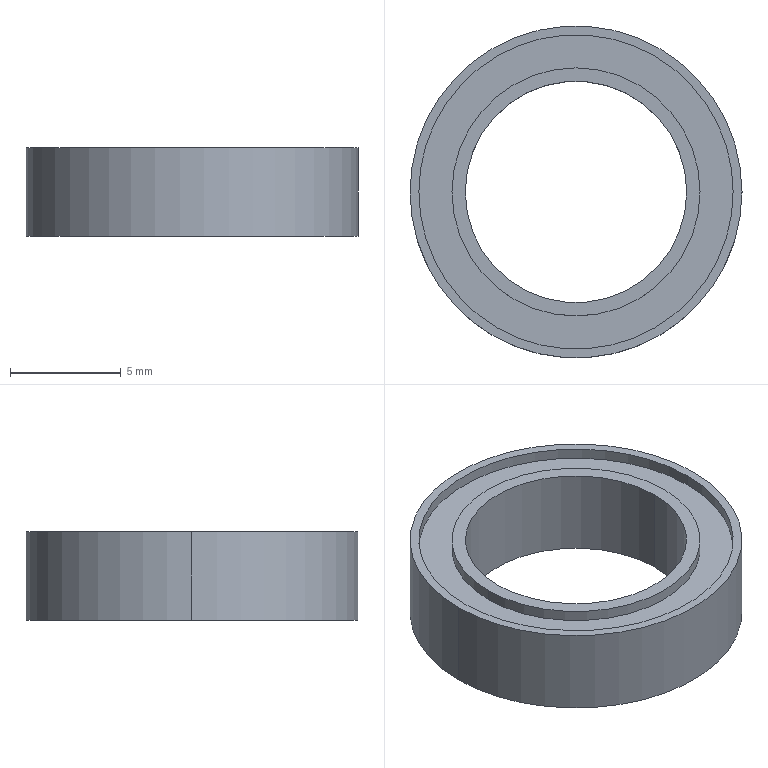Part | SolidWorks | features Extrusion 1, ICE 1, MirrorPattern 1 | 1 solid | 18 faces | box 15 x 15 x 4 mm | volume 333.028 mm3 | cylinder 12 | plane 6 | commonest cylinder face diameters 11.21 x4 14.2 x4 10 x2 15 x2
STEP:
#1=CARTESIAN_POINT('',(5.605,0.,-1.5));
#2=VERTEX_POINT('',#1);
#3=CARTESIAN_POINT('',(-5.605,0.,-1.5));
#4=VERTEX_POINT('',#3);
#5=CARTESIAN_POINT('',(0.,0.,-1.5));
#6=DIRECTION('',(0.,0.,1.));
#7=DIRECTION('',(1.,0.,0.));
#8=AXIS2_PLACEMENT_3D('',#5,#6,#7);
#9=CIRCLE('',#8,5.605);
#10=EDGE_CURVE('',#2,#4,#9,.T.);
#11=ORIENTED_EDGE('',*,*,#10,.F.);
#12=CARTESIAN_POINT('',(5.605,0.,-2.));
#13=VERTEX_POINT('',#12);
#14=CARTESIAN_POINT('',(5.605,0.,-1.5));
#15=DIRECTION('',(0.,0.,-1.));
#16=VECTOR('',#15,1000.);
#17=LINE('',#14,#16);
#18=EDGE_CURVE('',#2,#13,#17,.T.);
#19=ORIENTED_EDGE('',*,*,#18,.T.);
#20=CARTESIAN_POINT('',(-5.605,0.,-2.));
#21=VERTEX_POINT('',#20);
#22=CARTESIAN_POINT('',(0.,0.,-2.));
#23=DIRECTION('',(0.,0.,1.));
#24=DIRECTION('',(1.,0.,0.));
#25=AXIS2_PLACEMENT_3D('',#22,#23,#24);
#26=CIRCLE('',#25,5.605);
#27=EDGE_CURVE('',#13,#21,#26,.T.);
#28=ORIENTED_EDGE('',*,*,#27,.T.);
#29=CARTESIAN_POINT('',(-5.605,0.,-1.5));
#30=DIRECTION('',(0.,0.,-1.));
#31=VECTOR('',#30,1000.);
#32=LINE('',#29,#31);
#33=EDGE_CURVE('',#4,#21,#32,.T.);
#34=ORIENTED_EDGE('',*,*,#33,.F.);
#35=EDGE_LOOP('',(#11,#19,#28,#34));
#36=FACE_OUTER_BOUND('',#35,.T.);
#37=CARTESIAN_POINT('',(0.,0.,-1.5));
#38=DIRECTION('',(0.,0.,-1.));
#39=DIRECTION('',(-1.,0.,0.));
#40=AXIS2_PLACEMENT_3D('',#37,#38,#39);
#41=CYLINDRICAL_SURFACE('',#40,5.605);
#42=ADVANCED_FACE('',(#36),#41,.T.);
#43=CARTESIAN_POINT('',(-7.1,0.,-1.5));
#44=VERTEX_POINT('',#43);
#45=CARTESIAN_POINT('',(7.1,0.,-1.5));
#46=VERTEX_POINT('',#45);
#47=CARTESIAN_POINT('',(0.,0.,-1.5));
#48=DIRECTION('',(0.,0.,1.));
#49=DIRECTION('',(1.,0.,0.));
#50=AXIS2_PLACEMENT_3D('',#47,#48,#49);
#51=CIRCLE('',#50,7.1);
#52=EDGE_CURVE('',#44,#46,#51,.T.);
#53=ORIENTED_EDGE('',*,*,#52,.T.);
#54=CARTESIAN_POINT('',(7.1,0.,-2.));
#55=VERTEX_POINT('',#54);
#56=CARTESIAN_POINT('',(7.1,0.,-1.5));
#57=DIRECTION('',(0.,0.,-1.));
#58=VECTOR('',#57,1000.);
#59=LINE('',#56,#58);
#60=EDGE_CURVE('',#46,#55,#59,.T.);
#61=ORIENTED_EDGE('',*,*,#60,.T.);
#62=CARTESIAN_POINT('',(-7.1,0.,-2.));
#63=VERTEX_POINT('',#62);
#64=CARTESIAN_POINT('',(0.,0.,-2.));
#65=DIRECTION('',(0.,0.,1.));
#66=DIRECTION('',(1.,0.,0.));
#67=AXIS2_PLACEMENT_3D('',#64,#65,#66);
#68=CIRCLE('',#67,7.1);
#69=EDGE_CURVE('',#63,#55,#68,.T.);
#70=ORIENTED_EDGE('',*,*,#69,.F.);
#71=CARTESIAN_POINT('',(-7.1,0.,-1.5));
#72=DIRECTION('',(0.,0.,-1.));
#73=VECTOR('',#72,1000.);
#74=LINE('',#71,#73);
#75=EDGE_CURVE('',#44,#63,#74,.T.);
#76=ORIENTED_EDGE('',*,*,#75,.F.);
#77=EDGE_LOOP('',(#53,#61,#70,#76));
#78=FACE_OUTER_BOUND('',#77,.T.);
#79=CARTESIAN_POINT('',(0.,0.,-1.5));
#80=DIRECTION('',(0.,0.,-1.));
#81=DIRECTION('',(-1.,0.,0.));
#82=AXIS2_PLACEMENT_3D('',#79,#80,#81);
#83=CYLINDRICAL_SURFACE('',#82,7.1);
#84=ADVANCED_FACE('',(#78),#83,.F.);
#85=CARTESIAN_POINT('',(5.605,0.,1.5));
#86=VERTEX_POINT('',#85);
#87=CARTESIAN_POINT('',(-5.605,0.,1.5));
#88=VERTEX_POINT('',#87);
#89=CARTESIAN_POINT('',(0.,0.,1.5));
#90=DIRECTION('',(0.,0.,1.));
#91=DIRECTION('',(1.,0.,0.));
#92=AXIS2_PLACEMENT_3D('',#89,#90,#91);
#93=CIRCLE('',#92,5.605);
#94=EDGE_CURVE('',#86,#88,#93,.T.);
#95=ORIENTED_EDGE('',*,*,#94,.T.);
#96=CARTESIAN_POINT('',(-5.605,0.,2.));
#97=VERTEX_POINT('',#96);
#98=CARTESIAN_POINT('',(-5.605,0.,1.5));
#99=DIRECTION('',(0.,0.,1.));
#100=VECTOR('',#99,1000.);
#101=LINE('',#98,#100);
#102=EDGE_CURVE('',#88,#97,#101,.T.);
#103=ORIENTED_EDGE('',*,*,#102,.T.);
#104=CARTESIAN_POINT('',(5.605,0.,2.));
#105=VERTEX_POINT('',#104);
#106=CARTESIAN_POINT('',(0.,0.,2.));
#107=DIRECTION('',(0.,0.,1.));
#108=DIRECTION('',(1.,0.,0.));
#109=AXIS2_PLACEMENT_3D('',#106,#107,#108);
#110=CIRCLE('',#109,5.605);
#111=EDGE_CURVE('',#105,#97,#110,.T.);
#112=ORIENTED_EDGE('',*,*,#111,.F.);
#113=CARTESIAN_POINT('',(5.605,0.,1.5));
#114=DIRECTION('',(0.,0.,1.));
#115=VECTOR('',#114,1000.);
#116=LINE('',#113,#115);
#117=EDGE_CURVE('',#86,#105,#116,.T.);
#118=ORIENTED_EDGE('',*,*,#117,.F.);
#119=EDGE_LOOP('',(#95,#103,#112,#118));
#120=FACE_OUTER_BOUND('',#119,.T.);
#121=CARTESIAN_POINT('',(0.,0.,1.5));
#122=DIRECTION('',(0.,0.,1.));
#123=DIRECTION('',(1.,0.,0.));
#124=AXIS2_PLACEMENT_3D('',#121,#122,#123);
#125=CYLINDRICAL_SURFACE('',#124,5.605);
#126=ADVANCED_FACE('',(#120),#125,.T.);
#127=CARTESIAN_POINT('',(-7.1,0.,1.5));
#128=VERTEX_POINT('',#127);
#129=CARTESIAN_POINT('',(7.1,0.,1.5));
#130=VERTEX_POINT('',#129);
#131=CARTESIAN_POINT('',(0.,0.,1.5));
#132=DIRECTION('',(0.,0.,1.));
#133=DIRECTION('',(1.,0.,0.));
#134=AXIS2_PLACEMENT_3D('',#131,#132,#133);
#135=CIRCLE('',#134,7.1);
#136=EDGE_CURVE('',#128,#130,#135,.T.);
#137=ORIENTED_EDGE('',*,*,#136,.F.);
#138=CARTESIAN_POINT('',(-7.1,0.,2.));
#139=VERTEX_POINT('',#138);
#140=CARTESIAN_POINT('',(-7.1,0.,1.5));
#141=DIRECTION('',(0.,0.,1.));
#142=VECTOR('',#141,1000.);
#143=LINE('',#140,#142);
#144=EDGE_CURVE('',#128,#139,#143,.T.);
#145=ORIENTED_EDGE('',*,*,#144,.T.);
#146=CARTESIAN_POINT('',(7.1,0.,2.));
#147=VERTEX_POINT('',#146);
#148=CARTESIAN_POINT('',(0.,0.,2.));
#149=DIRECTION('',(0.,0.,1.));
#150=DIRECTION('',(1.,0.,0.));
#151=AXIS2_PLACEMENT_3D('',#148,#149,#150);
#152=CIRCLE('',#151,7.1);
#153=EDGE_CURVE('',#139,#147,#152,.T.);
#154=ORIENTED_EDGE('',*,*,#153,.T.);
#155=CARTESIAN_POINT('',(7.1,0.,1.5));
#156=DIRECTION('',(0.,0.,1.));
#157=VECTOR('',#156,1000.);
#158=LINE('',#155,#157);
#159=EDGE_CURVE('',#130,#147,#158,.T.);
#160=ORIENTED_EDGE('',*,*,#159,.F.);
#161=EDGE_LOOP('',(#137,#145,#154,#160));
#162=FACE_OUTER_BOUND('',#161,.T.);
#163=CARTESIAN_POINT('',(0.,0.,1.5));
#164=DIRECTION('',(0.,0.,1.));
#165=DIRECTION('',(1.,0.,0.));
#166=AXIS2_PLACEMENT_3D('',#163,#164,#165);
#167=CYLINDRICAL_SURFACE('',#166,7.1);
#168=ADVANCED_FACE('',(#162),#167,.F.);
#169=CARTESIAN_POINT('',(-5.,0.,-2.));
#170=VERTEX_POINT('',#169);
#171=CARTESIAN_POINT('',(5.,0.,-2.));
#172=VERTEX_POINT('',#171);
#173=CARTESIAN_POINT('',(0.,0.,-2.));
#174=DIRECTION('',(0.,0.,1.));
#175=DIRECTION('',(1.,0.,0.));
#176=AXIS2_PLACEMENT_3D('',#173,#174,#175);
#177=CIRCLE('',#176,5.);
#178=EDGE_CURVE('',#170,#172,#177,.T.);
#179=ORIENTED_EDGE('',*,*,#178,.F.);
#180=CARTESIAN_POINT('',(-5.,0.,2.));
#181=VERTEX_POINT('',#180);
#182=CARTESIAN_POINT('',(-5.,0.,-2.));
#183=DIRECTION('',(0.,0.,1.));
#184=VECTOR('',#183,1000.);
#185=LINE('',#182,#184);
#186=EDGE_CURVE('',#170,#181,#185,.T.);
#187=ORIENTED_EDGE('',*,*,#186,.T.);
#188=CARTESIAN_POINT('',(5.,0.,2.));
#189=VERTEX_POINT('',#188);
#190=CARTESIAN_POINT('',(0.,0.,2.));
#191=DIRECTION('',(0.,0.,1.));
#192=DIRECTION('',(1.,0.,0.));
#193=AXIS2_PLACEMENT_3D('',#190,#191,#192);
#194=CIRCLE('',#193,5.);
#195=EDGE_CURVE('',#181,#189,#194,.T.);
#196=ORIENTED_EDGE('',*,*,#195,.T.);
#197=CARTESIAN_POINT('',(5.,0.,-2.));
#198=DIRECTION('',(0.,0.,1.));
#199=VECTOR('',#198,1000.);
#200=LINE('',#197,#199);
#201=EDGE_CURVE('',#172,#189,#200,.T.);
#202=ORIENTED_EDGE('',*,*,#201,.F.);
#203=EDGE_LOOP('',(#179,#187,#196,#202));
#204=FACE_OUTER_BOUND('',#203,.T.);
#205=CARTESIAN_POINT('',(0.,0.,-2.));
#206=DIRECTION('',(0.,0.,1.));
#207=DIRECTION('',(1.,0.,0.));
#208=AXIS2_PLACEMENT_3D('',#205,#206,#207);
#209=CYLINDRICAL_SURFACE('',#208,5.);
#210=ADVANCED_FACE('',(#204),#209,.F.);
#211=CARTESIAN_POINT('',(7.5,0.,-2.));
#212=VERTEX_POINT('',#211);
#213=CARTESIAN_POINT('',(-7.5,0.,-2.));
#214=VERTEX_POINT('',#213);
#215=CARTESIAN_POINT('',(0.,0.,-2.));
#216=DIRECTION('',(0.,0.,1.));
#217=DIRECTION('',(1.,0.,0.));
#218=AXIS2_PLACEMENT_3D('',#215,#216,#217);
#219=CIRCLE('',#218,7.5);
#220=EDGE_CURVE('',#212,#214,#219,.T.);
#221=ORIENTED_EDGE('',*,*,#220,.T.);
#222=CARTESIAN_POINT('',(-7.5,0.,2.));
#223=VERTEX_POINT('',#222);
#224=CARTESIAN_POINT('',(-7.5,0.,-2.));
#225=DIRECTION('',(0.,0.,1.));
#226=VECTOR('',#225,1000.);
#227=LINE('',#224,#226);
#228=EDGE_CURVE('',#214,#223,#227,.T.);
#229=ORIENTED_EDGE('',*,*,#228,.T.);
#230=CARTESIAN_POINT('',(7.5,0.,2.));
#231=VERTEX_POINT('',#230);
#232=CARTESIAN_POINT('',(0.,0.,2.));
#233=DIRECTION('',(0.,0.,1.));
#234=DIRECTION('',(1.,0.,0.));
#235=AXIS2_PLACEMENT_3D('',#232,#233,#234);
#236=CIRCLE('',#235,7.5);
#237=EDGE_CURVE('',#231,#223,#236,.T.);
#238=ORIENTED_EDGE('',*,*,#237,.F.);
#239=CARTESIAN_POINT('',(7.5,0.,-2.));
#240=DIRECTION('',(0.,0.,1.));
#241=VECTOR('',#240,1000.);
#242=LINE('',#239,#241);
#243=EDGE_CURVE('',#212,#231,#242,.T.);
#244=ORIENTED_EDGE('',*,*,#243,.F.);
#245=EDGE_LOOP('',(#221,#229,#238,#244));
#246=FACE_OUTER_BOUND('',#245,.T.);
#247=CARTESIAN_POINT('',(0.,0.,-2.));
#248=DIRECTION('',(0.,0.,1.));
#249=DIRECTION('',(1.,0.,0.));
#250=AXIS2_PLACEMENT_3D('',#247,#248,#249);
#251=CYLINDRICAL_SURFACE('',#250,7.5);
#252=ADVANCED_FACE('',(#246),#251,.T.);
#253=ORIENTED_EDGE('',*,*,#220,.F.);
#254=CARTESIAN_POINT('',(0.,0.,-2.));
#255=DIRECTION('',(0.,0.,1.));
#256=DIRECTION('',(1.,0.,0.));
#257=AXIS2_PLACEMENT_3D('',#254,#255,#256);
#258=CIRCLE('',#257,7.5);
#259=EDGE_CURVE('',#214,#212,#258,.T.);
#260=ORIENTED_EDGE('',*,*,#259,.F.);
#261=EDGE_LOOP('',(#253,#260));
#262=FACE_OUTER_BOUND('',#261,.T.);
#263=ORIENTED_EDGE('',*,*,#69,.T.);
#264=CARTESIAN_POINT('',(0.,0.,-2.));
#265=DIRECTION('',(0.,0.,1.));
#266=DIRECTION('',(1.,0.,0.));
#267=AXIS2_PLACEMENT_3D('',#264,#265,#266);
#268=CIRCLE('',#267,7.1);
#269=EDGE_CURVE('',#55,#63,#268,.T.);
#270=ORIENTED_EDGE('',*,*,#269,.T.);
#271=EDGE_LOOP('',(#263,#270));
#272=FACE_BOUND('',#271,.T.);
#273=CARTESIAN_POINT('',(0.,0.,-2.));
#274=DIRECTION('',(0.,0.,1.));
#275=DIRECTION('',(1.,0.,0.));
#276=AXIS2_PLACEMENT_3D('',#273,#274,#275);
#277=PLANE('',#276);
#278=ADVANCED_FACE('',(#262,#272),#277,.F.);
#279=CARTESIAN_POINT('',(0.,0.,2.));
#280=DIRECTION('',(0.,0.,1.));
#281=DIRECTION('',(1.,0.,0.));
#282=AXIS2_PLACEMENT_3D('',#279,#280,#281);
#283=CIRCLE('',#282,5.);
#284=EDGE_CURVE('',#189,#181,#283,.T.);
#285=ORIENTED_EDGE('',*,*,#284,.F.);
#286=ORIENTED_EDGE('',*,*,#195,.F.);
#287=EDGE_LOOP('',(#285,#286));
#288=FACE_BOUND('',#287,.T.);
#289=ORIENTED_EDGE('',*,*,#111,.T.);
#290=CARTESIAN_POINT('',(0.,0.,2.));
#291=DIRECTION('',(0.,0.,1.));
#292=DIRECTION('',(1.,0.,0.));
#293=AXIS2_PLACEMENT_3D('',#290,#291,#292);
#294=CIRCLE('',#293,5.605);
#295=EDGE_CURVE('',#97,#105,#294,.T.);
#296=ORIENTED_EDGE('',*,*,#295,.T.);
#297=EDGE_LOOP('',(#289,#296));
#298=FACE_OUTER_BOUND('',#297,.T.);
#299=CARTESIAN_POINT('',(0.,0.,2.));
#300=DIRECTION('',(0.,0.,1.));
#301=DIRECTION('',(1.,0.,0.));
#302=AXIS2_PLACEMENT_3D('',#299,#300,#301);
#303=PLANE('',#302);
#304=ADVANCED_FACE('',(#288,#298),#303,.T.);
#305=ORIENTED_EDGE('',*,*,#228,.F.);
#306=ORIENTED_EDGE('',*,*,#259,.T.);
#307=ORIENTED_EDGE('',*,*,#243,.T.);
#308=CARTESIAN_POINT('',(0.,0.,2.));
#309=DIRECTION('',(0.,0.,1.));
#310=DIRECTION('',(1.,0.,0.));
#311=AXIS2_PLACEMENT_3D('',#308,#309,#310);
#312=CIRCLE('',#311,7.5);
#313=EDGE_CURVE('',#223,#231,#312,.T.);
#314=ORIENTED_EDGE('',*,*,#313,.F.);
#315=EDGE_LOOP('',(#305,#306,#307,#314));
#316=FACE_OUTER_BOUND('',#315,.T.);
#317=CARTESIAN_POINT('',(0.,0.,-2.));
#318=DIRECTION('',(0.,0.,1.));
#319=DIRECTION('',(1.,0.,0.));
#320=AXIS2_PLACEMENT_3D('',#317,#318,#319);
#321=CYLINDRICAL_SURFACE('',#320,7.5);
#322=ADVANCED_FACE('',(#316),#321,.T.);
#323=CARTESIAN_POINT('',(0.,0.,-2.));
#324=DIRECTION('',(0.,0.,1.));
#325=DIRECTION('',(1.,0.,0.));
#326=AXIS2_PLACEMENT_3D('',#323,#324,#325);
#327=CIRCLE('',#326,5.605);
#328=EDGE_CURVE('',#21,#13,#327,.T.);
#329=ORIENTED_EDGE('',*,*,#328,.F.);
#330=ORIENTED_EDGE('',*,*,#27,.F.);
#331=EDGE_LOOP('',(#329,#330));
#332=FACE_OUTER_BOUND('',#331,.T.);
#333=CARTESIAN_POINT('',(0.,0.,-2.));
#334=DIRECTION('',(0.,0.,1.));
#335=DIRECTION('',(1.,0.,0.));
#336=AXIS2_PLACEMENT_3D('',#333,#334,#335);
#337=CIRCLE('',#336,5.);
#338=EDGE_CURVE('',#172,#170,#337,.T.);
#339=ORIENTED_EDGE('',*,*,#338,.T.);
#340=ORIENTED_EDGE('',*,*,#178,.T.);
#341=EDGE_LOOP('',(#339,#340));
#342=FACE_BOUND('',#341,.T.);
#343=CARTESIAN_POINT('',(0.,0.,-2.));
#344=DIRECTION('',(0.,0.,1.));
#345=DIRECTION('',(1.,0.,0.));
#346=AXIS2_PLACEMENT_3D('',#343,#344,#345);
#347=PLANE('',#346);
#348=ADVANCED_FACE('',(#332,#342),#347,.F.);
#349=ORIENTED_EDGE('',*,*,#186,.F.);
#350=ORIENTED_EDGE('',*,*,#338,.F.);
#351=ORIENTED_EDGE('',*,*,#201,.T.);
#352=ORIENTED_EDGE('',*,*,#284,.T.);
#353=EDGE_LOOP('',(#349,#350,#351,#352));
#354=FACE_OUTER_BOUND('',#353,.T.);
#355=CARTESIAN_POINT('',(0.,0.,-2.));
#356=DIRECTION('',(0.,0.,1.));
#357=DIRECTION('',(1.,0.,0.));
#358=AXIS2_PLACEMENT_3D('',#355,#356,#357);
#359=CYLINDRICAL_SURFACE('',#358,5.);
#360=ADVANCED_FACE('',(#354),#359,.F.);
#361=CARTESIAN_POINT('',(0.,0.,2.));
#362=DIRECTION('',(0.,0.,1.));
#363=DIRECTION('',(1.,0.,0.));
#364=AXIS2_PLACEMENT_3D('',#361,#362,#363);
#365=CIRCLE('',#364,7.1);
#366=EDGE_CURVE('',#147,#139,#365,.T.);
#367=ORIENTED_EDGE('',*,*,#366,.F.);
#368=ORIENTED_EDGE('',*,*,#153,.F.);
#369=EDGE_LOOP('',(#367,#368));
#370=FACE_BOUND('',#369,.T.);
#371=ORIENTED_EDGE('',*,*,#237,.T.);
#372=ORIENTED_EDGE('',*,*,#313,.T.);
#373=EDGE_LOOP('',(#371,#372));
#374=FACE_OUTER_BOUND('',#373,.T.);
#375=CARTESIAN_POINT('',(0.,0.,2.));
#376=DIRECTION('',(0.,0.,1.));
#377=DIRECTION('',(1.,0.,0.));
#378=AXIS2_PLACEMENT_3D('',#375,#376,#377);
#379=PLANE('',#378);
#380=ADVANCED_FACE('',(#370,#374),#379,.T.);
#381=ORIENTED_EDGE('',*,*,#144,.F.);
#382=CARTESIAN_POINT('',(0.,0.,1.5));
#383=DIRECTION('',(0.,0.,1.));
#384=DIRECTION('',(1.,0.,0.));
#385=AXIS2_PLACEMENT_3D('',#382,#383,#384);
#386=CIRCLE('',#385,7.1);
#387=EDGE_CURVE('',#130,#128,#386,.T.);
#388=ORIENTED_EDGE('',*,*,#387,.F.);
#389=ORIENTED_EDGE('',*,*,#159,.T.);
#390=ORIENTED_EDGE('',*,*,#366,.T.);
#391=EDGE_LOOP('',(#381,#388,#389,#390));
#392=FACE_OUTER_BOUND('',#391,.T.);
#393=CARTESIAN_POINT('',(0.,0.,1.5));
#394=DIRECTION('',(0.,0.,1.));
#395=DIRECTION('',(1.,0.,0.));
#396=AXIS2_PLACEMENT_3D('',#393,#394,#395);
#397=CYLINDRICAL_SURFACE('',#396,7.1);
#398=ADVANCED_FACE('',(#392),#397,.F.);
#399=ORIENTED_EDGE('',*,*,#94,.F.);
#400=CARTESIAN_POINT('',(0.,0.,1.5));
#401=DIRECTION('',(0.,0.,1.));
#402=DIRECTION('',(1.,0.,0.));
#403=AXIS2_PLACEMENT_3D('',#400,#401,#402);
#404=CIRCLE('',#403,5.605);
#405=EDGE_CURVE('',#88,#86,#404,.T.);
#406=ORIENTED_EDGE('',*,*,#405,.F.);
#407=EDGE_LOOP('',(#399,#406));
#408=FACE_BOUND('',#407,.T.);
#409=ORIENTED_EDGE('',*,*,#387,.T.);
#410=ORIENTED_EDGE('',*,*,#136,.T.);
#411=EDGE_LOOP('',(#409,#410));
#412=FACE_OUTER_BOUND('',#411,.T.);
#413=CARTESIAN_POINT('',(0.,0.,1.5));
#414=DIRECTION('',(0.,0.,1.));
#415=DIRECTION('',(1.,0.,0.));
#416=AXIS2_PLACEMENT_3D('',#413,#414,#415);
#417=PLANE('',#416);
#418=ADVANCED_FACE('',(#408,#412),#417,.T.);
#419=ORIENTED_EDGE('',*,*,#102,.F.);
#420=ORIENTED_EDGE('',*,*,#405,.T.);
#421=ORIENTED_EDGE('',*,*,#117,.T.);
#422=ORIENTED_EDGE('',*,*,#295,.F.);
#423=EDGE_LOOP('',(#419,#420,#421,#422));
#424=FACE_OUTER_BOUND('',#423,.T.);
#425=CARTESIAN_POINT('',(0.,0.,1.5));
#426=DIRECTION('',(0.,0.,1.));
#427=DIRECTION('',(1.,0.,0.));
#428=AXIS2_PLACEMENT_3D('',#425,#426,#427);
#429=CYLINDRICAL_SURFACE('',#428,5.605);
#430=ADVANCED_FACE('',(#424),#429,.T.);
#431=ORIENTED_EDGE('',*,*,#52,.F.);
#432=CARTESIAN_POINT('',(0.,0.,-1.5));
#433=DIRECTION('',(0.,0.,1.));
#434=DIRECTION('',(1.,0.,0.));
#435=AXIS2_PLACEMENT_3D('',#432,#433,#434);
#436=CIRCLE('',#435,7.1);
#437=EDGE_CURVE('',#46,#44,#436,.T.);
#438=ORIENTED_EDGE('',*,*,#437,.F.);
#439=EDGE_LOOP('',(#431,#438));
#440=FACE_OUTER_BOUND('',#439,.T.);
#441=CARTESIAN_POINT('',(0.,0.,-1.5));
#442=DIRECTION('',(0.,0.,1.));
#443=DIRECTION('',(1.,0.,0.));
#444=AXIS2_PLACEMENT_3D('',#441,#442,#443);
#445=CIRCLE('',#444,5.605);
#446=EDGE_CURVE('',#4,#2,#445,.T.);
#447=ORIENTED_EDGE('',*,*,#446,.T.);
#448=ORIENTED_EDGE('',*,*,#10,.T.);
#449=EDGE_LOOP('',(#447,#448));
#450=FACE_BOUND('',#449,.T.);
#451=CARTESIAN_POINT('',(0.,0.,-1.5));
#452=DIRECTION('',(0.,0.,-1.));
#453=DIRECTION('',(1.,0.,0.));
#454=AXIS2_PLACEMENT_3D('',#451,#452,#453);
#455=PLANE('',#454);
#456=ADVANCED_FACE('',(#440,#450),#455,.T.);
#457=ORIENTED_EDGE('',*,*,#60,.F.);
#458=ORIENTED_EDGE('',*,*,#437,.T.);
#459=ORIENTED_EDGE('',*,*,#75,.T.);
#460=ORIENTED_EDGE('',*,*,#269,.F.);
#461=EDGE_LOOP('',(#457,#458,#459,#460));
#462=FACE_OUTER_BOUND('',#461,.T.);
#463=CARTESIAN_POINT('',(0.,0.,-1.5));
#464=DIRECTION('',(0.,0.,-1.));
#465=DIRECTION('',(-1.,0.,0.));
#466=AXIS2_PLACEMENT_3D('',#463,#464,#465);
#467=CYLINDRICAL_SURFACE('',#466,7.1);
#468=ADVANCED_FACE('',(#462),#467,.F.);
#469=ORIENTED_EDGE('',*,*,#18,.F.);
#470=ORIENTED_EDGE('',*,*,#446,.F.);
#471=ORIENTED_EDGE('',*,*,#33,.T.);
#472=ORIENTED_EDGE('',*,*,#328,.T.);
#473=EDGE_LOOP('',(#469,#470,#471,#472));
#474=FACE_OUTER_BOUND('',#473,.T.);
#475=CARTESIAN_POINT('',(0.,0.,-1.5));
#476=DIRECTION('',(0.,0.,-1.));
#477=DIRECTION('',(-1.,0.,0.));
#478=AXIS2_PLACEMENT_3D('',#475,#476,#477);
#479=CYLINDRICAL_SURFACE('',#478,5.605);
#480=ADVANCED_FACE('',(#474),#479,.T.);
#481=CLOSED_SHELL('',(#42,#84,#126,#168,#210,#252,#278,#304,#322,#348,#360,#380,#398,#418,#430,#456,#468,#480));
#482=MANIFOLD_SOLID_BREP('',#481);
#483=CARTESIAN_POINT('',(0.,0.,0.));
#484=DIRECTION('',(0.,0.,1.));
#485=DIRECTION('',(1.,0.,0.));
#486=AXIS2_PLACEMENT_3D('',#483,#484,#485);
#487=(LENGTH_UNIT()NAMED_UNIT(*)SI_UNIT(.MILLI.,.METRE.));
#488=UNCERTAINTY_MEASURE_WITH_UNIT(LENGTH_MEASURE(0.00001),#487,'','');
#489=(NAMED_UNIT(*)PLANE_ANGLE_UNIT()SI_UNIT($,.RADIAN.));
#490=(NAMED_UNIT(*)SI_UNIT($,.STERADIAN.)SOLID_ANGLE_UNIT());
#491=(GEOMETRIC_REPRESENTATION_CONTEXT(3)GLOBAL_UNCERTAINTY_ASSIGNED_CONTEXT((#488))GLOBAL_UNIT_ASSIGNED_CONTEXT((#487,#489,#490))REPRESENTATION_CONTEXT('',''));
#492=ADVANCED_BREP_SHAPE_REPRESENTATION('',(#482,#486),#491);